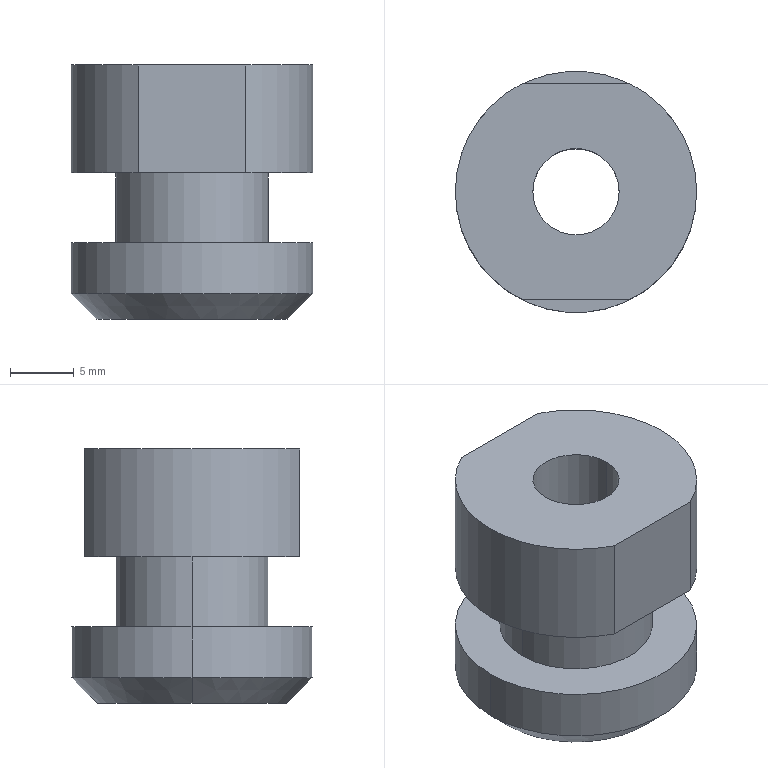Part | NX | 1 solid | 19 faces | box 19 x 19 x 20 mm | volume 3789 mm3 | cylinder 9 | plane 6 | cone 4 | commonest cylinder face diameters 19 x5 6.8 x2 12 x2
STEP:
#1=CARTESIAN_POINT('',(-94.033,-7.21,239.7));
#2=VERTEX_POINT('',#1);
#3=CARTESIAN_POINT('',(-94.033,-7.21,231.2));
#4=VERTEX_POINT('',#3);
#5=CARTESIAN_POINT('',(-94.033,-7.21,236.7));
#6=DIRECTION('',(0.,0.,-1.));
#7=VECTOR('',#6,1000.);
#8=LINE('',#5,#7);
#9=EDGE_CURVE('',#2,#4,#8,.T.);
#10=ORIENTED_EDGE('',*,*,#9,.F.);
#11=CARTESIAN_POINT('',(-99.29,-15.71,239.7));
#12=VERTEX_POINT('',#11);
#13=CARTESIAN_POINT('',(-103.533,-7.21,239.7));
#14=DIRECTION('',(0.,0.,1.));
#15=DIRECTION('',(1.,0.,0.));
#16=AXIS2_PLACEMENT_3D('',#13,#14,#15);
#17=CIRCLE('',#16,9.5);
#18=EDGE_CURVE('',#12,#2,#17,.T.);
#19=ORIENTED_EDGE('',*,*,#18,.F.);
#20=CARTESIAN_POINT('',(-99.29,-15.71,231.2));
#21=VERTEX_POINT('',#20);
#22=CARTESIAN_POINT('',(-99.29,-15.71,236.7));
#23=DIRECTION('',(0.,0.,-1.));
#24=VECTOR('',#23,1000.);
#25=LINE('',#22,#24);
#26=EDGE_CURVE('',#12,#21,#25,.T.);
#27=ORIENTED_EDGE('',*,*,#26,.T.);
#28=CARTESIAN_POINT('',(-103.533,-7.21,231.2));
#29=DIRECTION('',(0.,0.,1.));
#30=DIRECTION('',(1.,0.,0.));
#31=AXIS2_PLACEMENT_3D('',#28,#29,#30);
#32=CIRCLE('',#31,9.5);
#33=EDGE_CURVE('',#21,#4,#32,.T.);
#34=ORIENTED_EDGE('',*,*,#33,.T.);
#35=EDGE_LOOP('',(#10,#19,#27,#34));
#36=FACE_BOUND('',#35,.T.);
#37=CARTESIAN_POINT('',(-103.533,-7.21,236.7));
#38=DIRECTION('',(0.,0.,-1.));
#39=DIRECTION('',(1.,0.,0.));
#40=AXIS2_PLACEMENT_3D('',#37,#38,#39);
#41=CYLINDRICAL_SURFACE('',#40,9.5);
#42=ADVANCED_FACE('',(#36),#41,.T.);
#43=CARTESIAN_POINT('',(-107.775,1.29,231.2));
#44=VERTEX_POINT('',#43);
#45=CARTESIAN_POINT('',(-107.775,-15.71,231.2));
#46=VERTEX_POINT('',#45);
#47=CARTESIAN_POINT('',(-103.533,-7.21,231.2));
#48=DIRECTION('',(0.,0.,1.));
#49=DIRECTION('',(1.,0.,0.));
#50=AXIS2_PLACEMENT_3D('',#47,#48,#49);
#51=CIRCLE('',#50,9.5);
#52=EDGE_CURVE('',#44,#46,#51,.T.);
#53=ORIENTED_EDGE('',*,*,#52,.T.);
#54=CARTESIAN_POINT('',(-107.775,-15.71,239.7));
#55=VERTEX_POINT('',#54);
#56=CARTESIAN_POINT('',(-107.775,-15.71,236.7));
#57=DIRECTION('',(0.,0.,-1.));
#58=VECTOR('',#57,1000.);
#59=LINE('',#56,#58);
#60=EDGE_CURVE('',#55,#46,#59,.T.);
#61=ORIENTED_EDGE('',*,*,#60,.F.);
#62=CARTESIAN_POINT('',(-107.775,1.29,239.7));
#63=VERTEX_POINT('',#62);
#64=CARTESIAN_POINT('',(-103.533,-7.21,239.7));
#65=DIRECTION('',(0.,0.,1.));
#66=DIRECTION('',(1.,0.,0.));
#67=AXIS2_PLACEMENT_3D('',#64,#65,#66);
#68=CIRCLE('',#67,9.5);
#69=EDGE_CURVE('',#63,#55,#68,.T.);
#70=ORIENTED_EDGE('',*,*,#69,.F.);
#71=CARTESIAN_POINT('',(-107.775,1.29,236.7));
#72=DIRECTION('',(0.,0.,-1.));
#73=VECTOR('',#72,1000.);
#74=LINE('',#71,#73);
#75=EDGE_CURVE('',#63,#44,#74,.T.);
#76=ORIENTED_EDGE('',*,*,#75,.T.);
#77=EDGE_LOOP('',(#53,#61,#70,#76));
#78=FACE_BOUND('',#77,.T.);
#79=CARTESIAN_POINT('',(-103.533,-7.21,236.7));
#80=DIRECTION('',(0.,0.,-1.));
#81=DIRECTION('',(1.,0.,0.));
#82=AXIS2_PLACEMENT_3D('',#79,#80,#81);
#83=CYLINDRICAL_SURFACE('',#82,9.5);
#84=ADVANCED_FACE('',(#78),#83,.T.);
#85=ORIENTED_EDGE('',*,*,#60,.T.);
#86=CARTESIAN_POINT('',(0.,-15.71,231.2));
#87=DIRECTION('',(-1.,0.,0.));
#88=VECTOR('',#87,1000.);
#89=LINE('',#86,#88);
#90=EDGE_CURVE('',#21,#46,#89,.T.);
#91=ORIENTED_EDGE('',*,*,#90,.F.);
#92=ORIENTED_EDGE('',*,*,#26,.F.);
#93=CARTESIAN_POINT('',(0.,-15.71,239.7));
#94=DIRECTION('',(1.,0.,0.));
#95=VECTOR('',#94,1000.);
#96=LINE('',#93,#95);
#97=EDGE_CURVE('',#55,#12,#96,.T.);
#98=ORIENTED_EDGE('',*,*,#97,.F.);
#99=EDGE_LOOP('',(#85,#91,#92,#98));
#100=FACE_BOUND('',#99,.T.);
#101=CARTESIAN_POINT('',(-99.791,-15.71,236.7));
#102=DIRECTION('',(0.,1.,0.));
#103=DIRECTION('',(1.,0.,0.));
#104=AXIS2_PLACEMENT_3D('',#101,#102,#103);
#105=PLANE('',#104);
#106=ADVANCED_FACE('',(#100),#105,.F.);
#107=CARTESIAN_POINT('',(-108.095,-7.21,219.7));
#108=VERTEX_POINT('',#107);
#109=CARTESIAN_POINT('',(-98.97,-7.21,219.7));
#110=VERTEX_POINT('',#109);
#111=CARTESIAN_POINT('',(-103.533,-7.21,219.7));
#112=DIRECTION('',(0.,0.,-1.));
#113=DIRECTION('',(-1.,0.,0.));
#114=AXIS2_PLACEMENT_3D('',#111,#112,#113);
#115=CIRCLE('',#114,4.562);
#116=EDGE_CURVE('',#108,#110,#115,.T.);
#117=ORIENTED_EDGE('',*,*,#116,.T.);
#118=CARTESIAN_POINT('',(-100.133,-7.21,220.371));
#119=VERTEX_POINT('',#118);
#120=CARTESIAN_POINT('',(-100.133,-7.21,220.371));
#121=DIRECTION('',(0.866,0.,-0.5));
#122=VECTOR('',#121,1000.);
#123=LINE('',#120,#122);
#124=EDGE_CURVE('',#119,#110,#123,.T.);
#125=ORIENTED_EDGE('',*,*,#124,.F.);
#126=CARTESIAN_POINT('',(-106.933,-7.21,220.371));
#127=VERTEX_POINT('',#126);
#128=CARTESIAN_POINT('',(-103.533,-7.21,220.371));
#129=DIRECTION('',(0.,0.,-1.));
#130=DIRECTION('',(-1.,0.,0.));
#131=AXIS2_PLACEMENT_3D('',#128,#129,#130);
#132=CIRCLE('',#131,3.4);
#133=EDGE_CURVE('',#127,#119,#132,.T.);
#134=ORIENTED_EDGE('',*,*,#133,.F.);
#135=CARTESIAN_POINT('',(-106.933,-7.21,220.371));
#136=DIRECTION('',(-0.866,0.,-0.5));
#137=VECTOR('',#136,1000.);
#138=LINE('',#135,#137);
#139=EDGE_CURVE('',#127,#108,#138,.T.);
#140=ORIENTED_EDGE('',*,*,#139,.T.);
#141=EDGE_LOOP('',(#117,#125,#134,#140));
#142=FACE_BOUND('',#141,.T.);
#143=CARTESIAN_POINT('',(-103.533,-7.21,220.371));
#144=DIRECTION('',(0.,0.,-1.));
#145=DIRECTION('',(-1.,0.,0.));
#146=AXIS2_PLACEMENT_3D('',#143,#144,#145);
#147=CONICAL_SURFACE('',#146,3.4,1.047);
#148=ADVANCED_FACE('',(#142),#147,.F.);
#149=CARTESIAN_POINT('',(-99.29,1.29,239.7));
#150=VERTEX_POINT('',#149);
#151=CARTESIAN_POINT('',(0.,1.29,239.7));
#152=DIRECTION('',(-1.,0.,0.));
#153=VECTOR('',#152,1000.);
#154=LINE('',#151,#153);
#155=EDGE_CURVE('',#150,#63,#154,.T.);
#156=ORIENTED_EDGE('',*,*,#155,.T.);
#157=ORIENTED_EDGE('',*,*,#69,.T.);
#158=ORIENTED_EDGE('',*,*,#97,.T.);
#159=ORIENTED_EDGE('',*,*,#18,.T.);
#160=CARTESIAN_POINT('',(-103.533,-7.21,239.7));
#161=DIRECTION('',(0.,0.,1.));
#162=DIRECTION('',(1.,0.,0.));
#163=AXIS2_PLACEMENT_3D('',#160,#161,#162);
#164=CIRCLE('',#163,9.5);
#165=EDGE_CURVE('',#2,#150,#164,.T.);
#166=ORIENTED_EDGE('',*,*,#165,.T.);
#167=EDGE_LOOP('',(#156,#157,#158,#159,#166));
#168=FACE_BOUND('',#167,.T.);
#169=CARTESIAN_POINT('',(-100.133,-7.21,239.7));
#170=VERTEX_POINT('',#169);
#171=CARTESIAN_POINT('',(-106.933,-7.21,239.7));
#172=VERTEX_POINT('',#171);
#173=CARTESIAN_POINT('',(-103.533,-7.21,239.7));
#174=DIRECTION('',(0.,0.,-1.));
#175=DIRECTION('',(1.,0.,0.));
#176=AXIS2_PLACEMENT_3D('',#173,#174,#175);
#177=CIRCLE('',#176,3.4);
#178=EDGE_CURVE('',#170,#172,#177,.T.);
#179=ORIENTED_EDGE('',*,*,#178,.T.);
#180=CARTESIAN_POINT('',(-103.533,-7.21,239.7));
#181=DIRECTION('',(0.,0.,-1.));
#182=DIRECTION('',(1.,0.,0.));
#183=AXIS2_PLACEMENT_3D('',#180,#181,#182);
#184=CIRCLE('',#183,3.4);
#185=EDGE_CURVE('',#172,#170,#184,.T.);
#186=ORIENTED_EDGE('',*,*,#185,.T.);
#187=EDGE_LOOP('',(#179,#186));
#188=FACE_BOUND('',#187,.T.);
#189=CARTESIAN_POINT('',(-104.112,-7.022,239.7));
#190=DIRECTION('',(0.,0.,1.));
#191=DIRECTION('',(1.,0.,0.));
#192=AXIS2_PLACEMENT_3D('',#189,#190,#191);
#193=PLANE('',#192);
#194=ADVANCED_FACE('',(#168,#188),#193,.T.);
#195=CARTESIAN_POINT('',(-113.033,-7.21,225.7));
#196=VERTEX_POINT('',#195);
#197=CARTESIAN_POINT('',(-94.033,-7.21,225.7));
#198=VERTEX_POINT('',#197);
#199=CARTESIAN_POINT('',(-103.533,-7.21,225.7));
#200=DIRECTION('',(0.,0.,1.));
#201=DIRECTION('',(1.,0.,0.));
#202=AXIS2_PLACEMENT_3D('',#199,#200,#201);
#203=CIRCLE('',#202,9.5);
#204=EDGE_CURVE('',#196,#198,#203,.T.);
#205=ORIENTED_EDGE('',*,*,#204,.T.);
#206=CARTESIAN_POINT('',(-103.533,-7.21,225.7));
#207=DIRECTION('',(0.,0.,1.));
#208=DIRECTION('',(1.,0.,0.));
#209=AXIS2_PLACEMENT_3D('',#206,#207,#208);
#210=CIRCLE('',#209,9.5);
#211=EDGE_CURVE('',#198,#196,#210,.T.);
#212=ORIENTED_EDGE('',*,*,#211,.T.);
#213=EDGE_LOOP('',(#205,#212));
#214=FACE_BOUND('',#213,.T.);
#215=CARTESIAN_POINT('',(-109.533,-7.21,225.7));
#216=VERTEX_POINT('',#215);
#217=CARTESIAN_POINT('',(-97.533,-7.21,225.7));
#218=VERTEX_POINT('',#217);
#219=CARTESIAN_POINT('',(-103.533,-7.21,225.7));
#220=DIRECTION('',(0.,0.,1.));
#221=DIRECTION('',(1.,0.,0.));
#222=AXIS2_PLACEMENT_3D('',#219,#220,#221);
#223=CIRCLE('',#222,6.);
#224=EDGE_CURVE('',#216,#218,#223,.T.);
#225=ORIENTED_EDGE('',*,*,#224,.F.);
#226=CARTESIAN_POINT('',(-103.533,-7.21,225.7));
#227=DIRECTION('',(0.,0.,1.));
#228=DIRECTION('',(1.,0.,0.));
#229=AXIS2_PLACEMENT_3D('',#226,#227,#228);
#230=CIRCLE('',#229,6.);
#231=EDGE_CURVE('',#218,#216,#230,.T.);
#232=ORIENTED_EDGE('',*,*,#231,.F.);
#233=EDGE_LOOP('',(#225,#232));
#234=FACE_BOUND('',#233,.T.);
#235=CARTESIAN_POINT('',(-103.03,-7.592,225.7));
#236=DIRECTION('',(0.,0.,1.));
#237=DIRECTION('',(1.,0.,0.));
#238=AXIS2_PLACEMENT_3D('',#235,#236,#237);
#239=PLANE('',#238);
#240=ADVANCED_FACE('',(#214,#234),#239,.T.);
#241=CARTESIAN_POINT('',(-97.533,-7.21,231.2));
#242=VERTEX_POINT('',#241);
#243=CARTESIAN_POINT('',(-109.533,-7.21,231.2));
#244=VERTEX_POINT('',#243);
#245=CARTESIAN_POINT('',(-103.533,-7.21,231.2));
#246=DIRECTION('',(0.,0.,1.));
#247=DIRECTION('',(1.,0.,0.));
#248=AXIS2_PLACEMENT_3D('',#245,#246,#247);
#249=CIRCLE('',#248,6.);
#250=EDGE_CURVE('',#242,#244,#249,.T.);
#251=ORIENTED_EDGE('',*,*,#250,.F.);
#252=CARTESIAN_POINT('',(-97.533,-7.21,230.7));
#253=DIRECTION('',(0.,0.,-1.));
#254=VECTOR('',#253,1000.);
#255=LINE('',#252,#254);
#256=EDGE_CURVE('',#242,#218,#255,.T.);
#257=ORIENTED_EDGE('',*,*,#256,.T.);
#258=ORIENTED_EDGE('',*,*,#231,.T.);
#259=CARTESIAN_POINT('',(-109.533,-7.21,230.7));
#260=DIRECTION('',(0.,0.,-1.));
#261=VECTOR('',#260,1000.);
#262=LINE('',#259,#261);
#263=EDGE_CURVE('',#244,#216,#262,.T.);
#264=ORIENTED_EDGE('',*,*,#263,.F.);
#265=EDGE_LOOP('',(#251,#257,#258,#264));
#266=FACE_BOUND('',#265,.T.);
#267=CARTESIAN_POINT('',(-103.533,-7.21,230.7));
#268=DIRECTION('',(0.,0.,-1.));
#269=DIRECTION('',(1.,0.,0.));
#270=AXIS2_PLACEMENT_3D('',#267,#268,#269);
#271=CYLINDRICAL_SURFACE('',#270,6.);
#272=ADVANCED_FACE('',(#266),#271,.T.);
#273=CARTESIAN_POINT('',(-96.033,-7.21,219.7));
#274=VERTEX_POINT('',#273);
#275=CARTESIAN_POINT('',(-111.033,-7.21,219.7));
#276=VERTEX_POINT('',#275);
#277=CARTESIAN_POINT('',(-103.533,-7.21,219.7));
#278=DIRECTION('',(0.,0.,1.));
#279=DIRECTION('',(1.,0.,0.));
#280=AXIS2_PLACEMENT_3D('',#277,#278,#279);
#281=CIRCLE('',#280,7.5);
#282=EDGE_CURVE('',#274,#276,#281,.T.);
#283=ORIENTED_EDGE('',*,*,#282,.F.);
#284=CARTESIAN_POINT('',(-103.533,-7.21,219.7));
#285=DIRECTION('',(0.,0.,1.));
#286=DIRECTION('',(1.,0.,0.));
#287=AXIS2_PLACEMENT_3D('',#284,#285,#286);
#288=CIRCLE('',#287,7.5);
#289=EDGE_CURVE('',#276,#274,#288,.T.);
#290=ORIENTED_EDGE('',*,*,#289,.F.);
#291=EDGE_LOOP('',(#283,#290));
#292=FACE_BOUND('',#291,.T.);
#293=ORIENTED_EDGE('',*,*,#116,.F.);
#294=CARTESIAN_POINT('',(-103.533,-7.21,219.7));
#295=DIRECTION('',(0.,0.,-1.));
#296=DIRECTION('',(-1.,0.,0.));
#297=AXIS2_PLACEMENT_3D('',#294,#295,#296);
#298=CIRCLE('',#297,4.562);
#299=EDGE_CURVE('',#110,#108,#298,.T.);
#300=ORIENTED_EDGE('',*,*,#299,.F.);
#301=EDGE_LOOP('',(#293,#300));
#302=FACE_BOUND('',#301,.T.);
#303=CARTESIAN_POINT('',(-103.03,-7.592,219.7));
#304=DIRECTION('',(0.,0.,1.));
#305=DIRECTION('',(1.,0.,0.));
#306=AXIS2_PLACEMENT_3D('',#303,#304,#305);
#307=PLANE('',#306);
#308=ADVANCED_FACE('',(#292,#302),#307,.F.);
#309=CARTESIAN_POINT('',(-94.033,-7.21,221.7));
#310=VERTEX_POINT('',#309);
#311=CARTESIAN_POINT('',(-113.033,-7.21,221.7));
#312=VERTEX_POINT('',#311);
#313=CARTESIAN_POINT('',(-103.533,-7.21,221.7));
#314=DIRECTION('',(0.,0.,1.));
#315=DIRECTION('',(1.,0.,0.));
#316=AXIS2_PLACEMENT_3D('',#313,#314,#315);
#317=CIRCLE('',#316,9.5);
#318=EDGE_CURVE('',#310,#312,#317,.T.);
#319=ORIENTED_EDGE('',*,*,#318,.T.);
#320=CARTESIAN_POINT('',(-113.033,-7.21,225.7));
#321=DIRECTION('',(0.,0.,-1.));
#322=VECTOR('',#321,1000.);
#323=LINE('',#320,#322);
#324=EDGE_CURVE('',#312,#196,#323,.F.);
#325=ORIENTED_EDGE('',*,*,#324,.T.);
#326=ORIENTED_EDGE('',*,*,#211,.F.);
#327=CARTESIAN_POINT('',(-94.033,-7.21,225.7));
#328=DIRECTION('',(0.,0.,-1.));
#329=VECTOR('',#328,1000.);
#330=LINE('',#327,#329);
#331=EDGE_CURVE('',#310,#198,#330,.F.);
#332=ORIENTED_EDGE('',*,*,#331,.F.);
#333=EDGE_LOOP('',(#319,#325,#326,#332));
#334=FACE_BOUND('',#333,.T.);
#335=CARTESIAN_POINT('',(-103.533,-7.21,225.7));
#336=DIRECTION('',(0.,0.,-1.));
#337=DIRECTION('',(1.,0.,0.));
#338=AXIS2_PLACEMENT_3D('',#335,#336,#337);
#339=CYLINDRICAL_SURFACE('',#338,9.5);
#340=ADVANCED_FACE('',(#334),#339,.T.);
#341=ORIENTED_EDGE('',*,*,#90,.T.);
#342=ORIENTED_EDGE('',*,*,#52,.F.);
#343=CARTESIAN_POINT('',(-99.29,1.29,231.2));
#344=VERTEX_POINT('',#343);
#345=CARTESIAN_POINT('',(0.,1.29,231.2));
#346=DIRECTION('',(1.,0.,0.));
#347=VECTOR('',#346,1000.);
#348=LINE('',#345,#347);
#349=EDGE_CURVE('',#44,#344,#348,.T.);
#350=ORIENTED_EDGE('',*,*,#349,.T.);
#351=CARTESIAN_POINT('',(-103.533,-7.21,231.2));
#352=DIRECTION('',(0.,0.,1.));
#353=DIRECTION('',(1.,0.,0.));
#354=AXIS2_PLACEMENT_3D('',#351,#352,#353);
#355=CIRCLE('',#354,9.5);
#356=EDGE_CURVE('',#4,#344,#355,.T.);
#357=ORIENTED_EDGE('',*,*,#356,.F.);
#358=ORIENTED_EDGE('',*,*,#33,.F.);
#359=EDGE_LOOP('',(#341,#342,#350,#357,#358));
#360=FACE_BOUND('',#359,.T.);
#361=ORIENTED_EDGE('',*,*,#250,.T.);
#362=CARTESIAN_POINT('',(-103.533,-7.21,231.2));
#363=DIRECTION('',(0.,0.,1.));
#364=DIRECTION('',(1.,0.,0.));
#365=AXIS2_PLACEMENT_3D('',#362,#363,#364);
#366=CIRCLE('',#365,6.);
#367=EDGE_CURVE('',#244,#242,#366,.T.);
#368=ORIENTED_EDGE('',*,*,#367,.T.);
#369=EDGE_LOOP('',(#361,#368));
#370=FACE_BOUND('',#369,.T.);
#371=CARTESIAN_POINT('',(-104.112,-7.022,231.2));
#372=DIRECTION('',(0.,0.,1.));
#373=DIRECTION('',(1.,0.,0.));
#374=AXIS2_PLACEMENT_3D('',#371,#372,#373);
#375=PLANE('',#374);
#376=ADVANCED_FACE('',(#360,#370),#375,.F.);
#377=CARTESIAN_POINT('',(-103.533,-7.21,220.371));
#378=DIRECTION('',(0.,0.,-1.));
#379=DIRECTION('',(-1.,0.,0.));
#380=AXIS2_PLACEMENT_3D('',#377,#378,#379);
#381=CIRCLE('',#380,3.4);
#382=EDGE_CURVE('',#119,#127,#381,.T.);
#383=ORIENTED_EDGE('',*,*,#382,.T.);
#384=CARTESIAN_POINT('',(-106.933,-7.21,228.7));
#385=DIRECTION('',(0.,0.,-1.));
#386=VECTOR('',#385,1000.);
#387=LINE('',#384,#386);
#388=EDGE_CURVE('',#172,#127,#387,.T.);
#389=ORIENTED_EDGE('',*,*,#388,.F.);
#390=ORIENTED_EDGE('',*,*,#178,.F.);
#391=CARTESIAN_POINT('',(-100.133,-7.21,228.7));
#392=DIRECTION('',(0.,0.,-1.));
#393=VECTOR('',#392,1000.);
#394=LINE('',#391,#393);
#395=EDGE_CURVE('',#170,#119,#394,.T.);
#396=ORIENTED_EDGE('',*,*,#395,.T.);
#397=EDGE_LOOP('',(#383,#389,#390,#396));
#398=FACE_BOUND('',#397,.T.);
#399=CARTESIAN_POINT('',(-103.533,-7.21,228.7));
#400=DIRECTION('',(0.,0.,-1.));
#401=DIRECTION('',(1.,0.,0.));
#402=AXIS2_PLACEMENT_3D('',#399,#400,#401);
#403=CYLINDRICAL_SURFACE('',#402,3.4);
#404=ADVANCED_FACE('',(#398),#403,.F.);
#405=CARTESIAN_POINT('',(-99.29,1.29,236.7));
#406=DIRECTION('',(0.,0.,-1.));
#407=VECTOR('',#406,1000.);
#408=LINE('',#405,#407);
#409=EDGE_CURVE('',#150,#344,#408,.T.);
#410=ORIENTED_EDGE('',*,*,#409,.T.);
#411=ORIENTED_EDGE('',*,*,#349,.F.);
#412=ORIENTED_EDGE('',*,*,#75,.F.);
#413=ORIENTED_EDGE('',*,*,#155,.F.);
#414=EDGE_LOOP('',(#410,#411,#412,#413));
#415=FACE_BOUND('',#414,.T.);
#416=CARTESIAN_POINT('',(-107.274,1.29,236.7));
#417=DIRECTION('',(0.,-1.,0.));
#418=DIRECTION('',(0.,0.,-1.));
#419=AXIS2_PLACEMENT_3D('',#416,#417,#418);
#420=PLANE('',#419);
#421=ADVANCED_FACE('',(#415),#420,.F.);
#422=ORIENTED_EDGE('',*,*,#282,.T.);
#423=CARTESIAN_POINT('',(-111.033,-7.21,219.7));
#424=DIRECTION('',(-0.7071,0.,0.7071));
#425=VECTOR('',#424,1000.);
#426=LINE('',#423,#425);
#427=EDGE_CURVE('',#276,#312,#426,.T.);
#428=ORIENTED_EDGE('',*,*,#427,.T.);
#429=ORIENTED_EDGE('',*,*,#318,.F.);
#430=CARTESIAN_POINT('',(-96.033,-7.21,219.7));
#431=DIRECTION('',(0.7071,0.,0.7071));
#432=VECTOR('',#431,1000.);
#433=LINE('',#430,#432);
#434=EDGE_CURVE('',#274,#310,#433,.T.);
#435=ORIENTED_EDGE('',*,*,#434,.F.);
#436=EDGE_LOOP('',(#422,#428,#429,#435));
#437=FACE_BOUND('',#436,.T.);
#438=CARTESIAN_POINT('',(-103.533,-7.21,219.7));
#439=DIRECTION('',(0.,0.,1.));
#440=DIRECTION('',(1.,0.,0.));
#441=AXIS2_PLACEMENT_3D('',#438,#439,#440);
#442=CONICAL_SURFACE('',#441,7.5,0.7854);
#443=ADVANCED_FACE('',(#437),#442,.T.);
#444=ORIENTED_EDGE('',*,*,#224,.T.);
#445=ORIENTED_EDGE('',*,*,#256,.F.);
#446=ORIENTED_EDGE('',*,*,#367,.F.);
#447=ORIENTED_EDGE('',*,*,#263,.T.);
#448=EDGE_LOOP('',(#444,#445,#446,#447));
#449=FACE_BOUND('',#448,.T.);
#450=CARTESIAN_POINT('',(-103.533,-7.21,230.7));
#451=DIRECTION('',(0.,0.,-1.));
#452=DIRECTION('',(1.,0.,0.));
#453=AXIS2_PLACEMENT_3D('',#450,#451,#452);
#454=CYLINDRICAL_SURFACE('',#453,6.);
#455=ADVANCED_FACE('',(#449),#454,.T.);
#456=ORIENTED_EDGE('',*,*,#395,.F.);
#457=ORIENTED_EDGE('',*,*,#185,.F.);
#458=ORIENTED_EDGE('',*,*,#388,.T.);
#459=ORIENTED_EDGE('',*,*,#133,.T.);
#460=EDGE_LOOP('',(#456,#457,#458,#459));
#461=FACE_BOUND('',#460,.T.);
#462=CARTESIAN_POINT('',(-103.533,-7.21,228.7));
#463=DIRECTION('',(0.,0.,-1.));
#464=DIRECTION('',(1.,0.,0.));
#465=AXIS2_PLACEMENT_3D('',#462,#463,#464);
#466=CYLINDRICAL_SURFACE('',#465,3.4);
#467=ADVANCED_FACE('',(#461),#466,.F.);
#468=ORIENTED_EDGE('',*,*,#382,.F.);
#469=ORIENTED_EDGE('',*,*,#124,.T.);
#470=ORIENTED_EDGE('',*,*,#299,.T.);
#471=ORIENTED_EDGE('',*,*,#139,.F.);
#472=EDGE_LOOP('',(#468,#469,#470,#471));
#473=FACE_BOUND('',#472,.T.);
#474=CARTESIAN_POINT('',(-103.533,-7.21,220.371));
#475=DIRECTION('',(0.,0.,-1.));
#476=DIRECTION('',(-1.,0.,0.));
#477=AXIS2_PLACEMENT_3D('',#474,#475,#476);
#478=CONICAL_SURFACE('',#477,3.4,1.047);
#479=ADVANCED_FACE('',(#473),#478,.F.);
#480=ORIENTED_EDGE('',*,*,#434,.T.);
#481=CARTESIAN_POINT('',(-103.533,-7.21,221.7));
#482=DIRECTION('',(0.,0.,1.));
#483=DIRECTION('',(1.,0.,0.));
#484=AXIS2_PLACEMENT_3D('',#481,#482,#483);
#485=CIRCLE('',#484,9.5);
#486=EDGE_CURVE('',#312,#310,#485,.T.);
#487=ORIENTED_EDGE('',*,*,#486,.F.);
#488=ORIENTED_EDGE('',*,*,#427,.F.);
#489=ORIENTED_EDGE('',*,*,#289,.T.);
#490=EDGE_LOOP('',(#480,#487,#488,#489));
#491=FACE_BOUND('',#490,.T.);
#492=CARTESIAN_POINT('',(-103.533,-7.21,219.7));
#493=DIRECTION('',(0.,0.,1.));
#494=DIRECTION('',(1.,0.,0.));
#495=AXIS2_PLACEMENT_3D('',#492,#493,#494);
#496=CONICAL_SURFACE('',#495,7.5,0.7854);
#497=ADVANCED_FACE('',(#491),#496,.T.);
#498=ORIENTED_EDGE('',*,*,#204,.F.);
#499=ORIENTED_EDGE('',*,*,#324,.F.);
#500=ORIENTED_EDGE('',*,*,#486,.T.);
#501=ORIENTED_EDGE('',*,*,#331,.T.);
#502=EDGE_LOOP('',(#498,#499,#500,#501));
#503=FACE_BOUND('',#502,.T.);
#504=CARTESIAN_POINT('',(-103.533,-7.21,225.7));
#505=DIRECTION('',(0.,0.,-1.));
#506=DIRECTION('',(1.,0.,0.));
#507=AXIS2_PLACEMENT_3D('',#504,#505,#506);
#508=CYLINDRICAL_SURFACE('',#507,9.5);
#509=ADVANCED_FACE('',(#503),#508,.T.);
#510=ORIENTED_EDGE('',*,*,#165,.F.);
#511=ORIENTED_EDGE('',*,*,#9,.T.);
#512=ORIENTED_EDGE('',*,*,#356,.T.);
#513=ORIENTED_EDGE('',*,*,#409,.F.);
#514=EDGE_LOOP('',(#510,#511,#512,#513));
#515=FACE_BOUND('',#514,.T.);
#516=CARTESIAN_POINT('',(-103.533,-7.21,236.7));
#517=DIRECTION('',(0.,0.,-1.));
#518=DIRECTION('',(1.,0.,0.));
#519=AXIS2_PLACEMENT_3D('',#516,#517,#518);
#520=CYLINDRICAL_SURFACE('',#519,9.5);
#521=ADVANCED_FACE('',(#515),#520,.T.);
#522=CLOSED_SHELL('',(#42,#84,#106,#148,#194,#240,#272,#308,#340,#376,#404,#421,#443,#455,#467,#479,#497,#509,#521));
#523=MANIFOLD_SOLID_BREP('',#522);
#524=(LENGTH_UNIT()NAMED_UNIT(*)SI_UNIT(.MILLI.,.METRE.));
#525=UNCERTAINTY_MEASURE_WITH_UNIT(LENGTH_MEASURE(0.00001),#524,'','');
#526=(NAMED_UNIT(*)PLANE_ANGLE_UNIT()SI_UNIT($,.RADIAN.));
#527=(NAMED_UNIT(*)SI_UNIT($,.STERADIAN.)SOLID_ANGLE_UNIT());
#528=(GEOMETRIC_REPRESENTATION_CONTEXT(3)GLOBAL_UNCERTAINTY_ASSIGNED_CONTEXT((#525))GLOBAL_UNIT_ASSIGNED_CONTEXT((#524,#526,#527))REPRESENTATION_CONTEXT('',''));
#529=ADVANCED_BREP_SHAPE_REPRESENTATION('',(#523),#528);